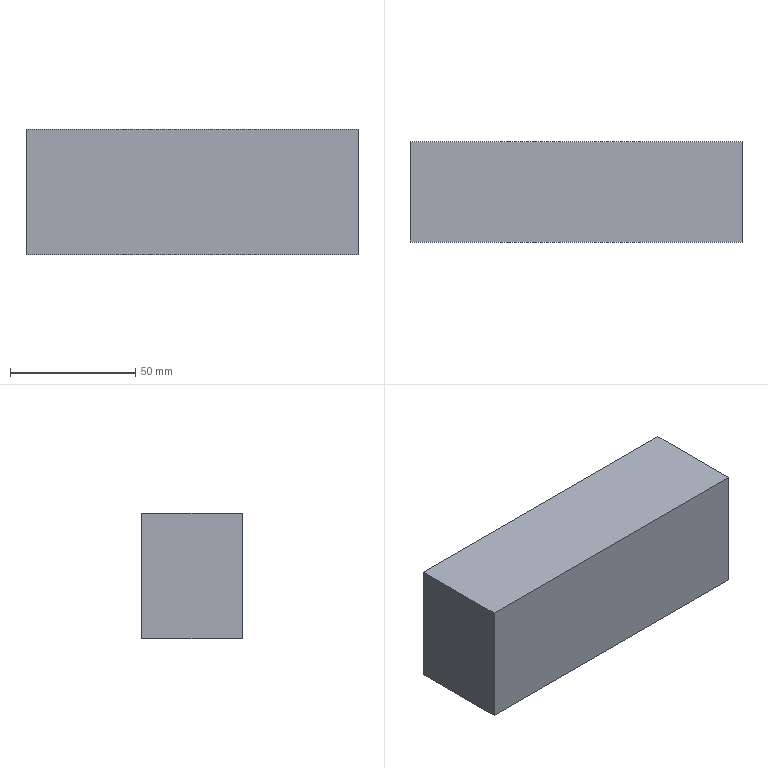Part | NX | features solid 2 | 1 solid | 6 faces | box 132.5 x 40 x 50 mm | volume 265000 mm3 | plane 4 | spline 2
STEP:
#1=CARTESIAN_POINT('',(402.5,390.,70.));
#2=VERTEX_POINT('',#1);
#3=CARTESIAN_POINT('',(270.,390.,70.));
#4=VERTEX_POINT('',#3);
#5=CARTESIAN_POINT('',(402.5,390.,70.));
#6=CARTESIAN_POINT('',(358.333,390.,70.));
#7=CARTESIAN_POINT('',(314.167,390.,70.));
#8=CARTESIAN_POINT('',(270.,390.,70.));
#9=B_SPLINE_CURVE_WITH_KNOTS('',3,(#5,#6,#7,#8),.UNSPECIFIED.,.F.,.F.,(4,4),(0.8545,0.987),.UNSPECIFIED.);
#10=EDGE_CURVE('',#2,#4,#9,.T.);
#11=ORIENTED_EDGE('',*,*,#10,.F.);
#12=CARTESIAN_POINT('',(402.5,390.,20.));
#13=VERTEX_POINT('',#12);
#14=CARTESIAN_POINT('',(402.5,390.,20.));
#15=DIRECTION('',(0.,0.,1.));
#16=VECTOR('',#15,1000.);
#17=LINE('',#14,#16);
#18=EDGE_CURVE('',#13,#2,#17,.T.);
#19=ORIENTED_EDGE('',*,*,#18,.F.);
#20=CARTESIAN_POINT('',(270.,390.,20.));
#21=VERTEX_POINT('',#20);
#22=CARTESIAN_POINT('',(402.5,390.,20.));
#23=CARTESIAN_POINT('',(358.333,390.,20.));
#24=CARTESIAN_POINT('',(314.167,390.,20.));
#25=CARTESIAN_POINT('',(270.,390.,20.));
#26=B_SPLINE_CURVE_WITH_KNOTS('',3,(#22,#23,#24,#25),.UNSPECIFIED.,.F.,.F.,(4,4),(0.8545,0.987),.UNSPECIFIED.);
#27=EDGE_CURVE('',#13,#21,#26,.T.);
#28=ORIENTED_EDGE('',*,*,#27,.T.);
#29=CARTESIAN_POINT('',(270.,390.,20.));
#30=DIRECTION('',(0.,0.,1.));
#31=VECTOR('',#30,1000.);
#32=LINE('',#29,#31);
#33=EDGE_CURVE('',#21,#4,#32,.T.);
#34=ORIENTED_EDGE('',*,*,#33,.T.);
#35=EDGE_LOOP('',(#11,#19,#28,#34));
#36=FACE_BOUND('',#35,.T.);
#37=CARTESIAN_POINT('',(442.5,390.,20.));
#38=DIRECTION('',(0.,1.,0.));
#39=DIRECTION('',(-1.,0.,0.));
#40=AXIS2_PLACEMENT_3D('',#37,#38,#39);
#41=PLANE('',#40);
#42=ADVANCED_FACE('',(#36),#41,.T.);
#43=CARTESIAN_POINT('',(270.,350.,70.));
#44=VERTEX_POINT('',#43);
#45=CARTESIAN_POINT('',(270.,490.534,70.));
#46=DIRECTION('',(0.,-1.,0.));
#47=VECTOR('',#46,1000.);
#48=LINE('',#45,#47);
#49=EDGE_CURVE('',#4,#44,#48,.T.);
#50=ORIENTED_EDGE('',*,*,#49,.F.);
#51=ORIENTED_EDGE('',*,*,#33,.F.);
#52=CARTESIAN_POINT('',(270.,350.,20.));
#53=VERTEX_POINT('',#52);
#54=CARTESIAN_POINT('',(270.,490.534,20.));
#55=DIRECTION('',(0.,-1.,0.));
#56=VECTOR('',#55,1000.);
#57=LINE('',#54,#56);
#58=EDGE_CURVE('',#21,#53,#57,.T.);
#59=ORIENTED_EDGE('',*,*,#58,.T.);
#60=CARTESIAN_POINT('',(270.,350.,20.));
#61=DIRECTION('',(0.,0.,1.));
#62=VECTOR('',#61,1000.);
#63=LINE('',#60,#62);
#64=EDGE_CURVE('',#53,#44,#63,.T.);
#65=ORIENTED_EDGE('',*,*,#64,.T.);
#66=EDGE_LOOP('',(#50,#51,#59,#65));
#67=FACE_BOUND('',#66,.T.);
#68=CARTESIAN_POINT('',(270.,490.534,20.));
#69=DIRECTION('',(-1.,0.,0.));
#70=DIRECTION('',(0.,0.,1.));
#71=AXIS2_PLACEMENT_3D('',#68,#69,#70);
#72=PLANE('',#71);
#73=ADVANCED_FACE('',(#67),#72,.T.);
#74=CARTESIAN_POINT('',(402.5,350.,70.));
#75=VERTEX_POINT('',#74);
#76=CARTESIAN_POINT('',(270.,350.,70.));
#77=CARTESIAN_POINT('',(314.167,350.,70.));
#78=CARTESIAN_POINT('',(358.333,350.,70.));
#79=CARTESIAN_POINT('',(402.5,350.,70.));
#80=B_SPLINE_CURVE_WITH_KNOTS('',3,(#76,#77,#78,#79),.UNSPECIFIED.,.F.,.F.,(4,4),(2.79,2.922),.UNSPECIFIED.);
#81=EDGE_CURVE('',#75,#44,#80,.F.);
#82=ORIENTED_EDGE('',*,*,#81,.T.);
#83=ORIENTED_EDGE('',*,*,#64,.F.);
#84=CARTESIAN_POINT('',(402.5,350.,20.));
#85=VERTEX_POINT('',#84);
#86=CARTESIAN_POINT('',(270.,350.,20.));
#87=CARTESIAN_POINT('',(314.167,350.,20.));
#88=CARTESIAN_POINT('',(358.333,350.,20.));
#89=CARTESIAN_POINT('',(402.5,350.,20.));
#90=B_SPLINE_CURVE_WITH_KNOTS('',3,(#86,#87,#88,#89),.UNSPECIFIED.,.F.,.F.,(4,4),(2.79,2.922),.UNSPECIFIED.);
#91=EDGE_CURVE('',#85,#53,#90,.F.);
#92=ORIENTED_EDGE('',*,*,#91,.F.);
#93=CARTESIAN_POINT('',(402.5,350.,20.));
#94=DIRECTION('',(0.,0.,1.));
#95=VECTOR('',#94,1000.);
#96=LINE('',#93,#95);
#97=EDGE_CURVE('',#85,#75,#96,.T.);
#98=ORIENTED_EDGE('',*,*,#97,.T.);
#99=EDGE_LOOP('',(#82,#83,#92,#98));
#100=FACE_BOUND('',#99,.T.);
#101=CARTESIAN_POINT('',(-270.,350.,20.));
#102=DIRECTION('',(0.,1.,0.));
#103=DIRECTION('',(0.,0.,1.));
#104=AXIS2_PLACEMENT_3D('',#101,#102,#103);
#105=PLANE('',#104);
#106=ADVANCED_FACE('',(#100),#105,.F.);
#107=CARTESIAN_POINT('',(402.5,350.,70.));
#108=CARTESIAN_POINT('',(402.5,363.333,70.));
#109=CARTESIAN_POINT('',(402.5,376.667,70.));
#110=CARTESIAN_POINT('',(402.5,390.,70.));
#111=B_SPLINE_CURVE_WITH_KNOTS('',3,(#107,#108,#109,#110),.UNSPECIFIED.,.F.,.F.,(4,4),(0.4214,0.4614),.UNSPECIFIED.);
#112=EDGE_CURVE('',#75,#2,#111,.T.);
#113=ORIENTED_EDGE('',*,*,#112,.F.);
#114=ORIENTED_EDGE('',*,*,#97,.F.);
#115=CARTESIAN_POINT('',(402.5,350.,20.));
#116=CARTESIAN_POINT('',(402.5,363.333,20.));
#117=CARTESIAN_POINT('',(402.5,376.667,20.));
#118=CARTESIAN_POINT('',(402.5,390.,20.));
#119=B_SPLINE_CURVE_WITH_KNOTS('',3,(#115,#116,#117,#118),.UNSPECIFIED.,.F.,.F.,(4,4),(0.4214,0.4614),.UNSPECIFIED.);
#120=EDGE_CURVE('',#85,#13,#119,.T.);
#121=ORIENTED_EDGE('',*,*,#120,.T.);
#122=ORIENTED_EDGE('',*,*,#18,.T.);
#123=EDGE_LOOP('',(#113,#114,#121,#122));
#124=FACE_BOUND('',#123,.T.);
#125=CARTESIAN_POINT('',(402.5,259.64,20.));
#126=DIRECTION('',(1.,0.,0.));
#127=DIRECTION('',(0.,0.,-1.));
#128=AXIS2_PLACEMENT_3D('',#125,#126,#127);
#129=PLANE('',#128);
#130=ADVANCED_FACE('',(#124),#129,.T.);
#131=ORIENTED_EDGE('',*,*,#27,.F.);
#132=ORIENTED_EDGE('',*,*,#120,.F.);
#133=ORIENTED_EDGE('',*,*,#91,.T.);
#134=ORIENTED_EDGE('',*,*,#58,.F.);
#135=EDGE_LOOP('',(#131,#132,#133,#134));
#136=FACE_BOUND('',#135,.T.);
#137=CARTESIAN_POINT('',(402.5,350.,20.));
#138=CARTESIAN_POINT('',(280.,350.,20.));
#139=CARTESIAN_POINT('',(270.,350.,20.));
#140=CARTESIAN_POINT('',(402.5,390.,20.));
#141=CARTESIAN_POINT('',(280.,390.,20.));
#142=CARTESIAN_POINT('',(270.,390.,20.));
#143=B_SPLINE_SURFACE_WITH_KNOTS('',1,1,((#137,#138,#139),(#140,#141,#142)),.PLANE_SURF.,.F.,.F.,.F.,(2,2),(2,1,2),(0.1041,0.2082),(-0.2188,0.,0.01786),.PIECEWISE_BEZIER_KNOTS.);
#144=ADVANCED_FACE('',(#136),#143,.F.);
#145=ORIENTED_EDGE('',*,*,#10,.T.);
#146=ORIENTED_EDGE('',*,*,#49,.T.);
#147=ORIENTED_EDGE('',*,*,#81,.F.);
#148=ORIENTED_EDGE('',*,*,#112,.T.);
#149=EDGE_LOOP('',(#145,#146,#147,#148));
#150=FACE_BOUND('',#149,.T.);
#151=CARTESIAN_POINT('',(402.5,350.,70.));
#152=CARTESIAN_POINT('',(280.,350.,70.));
#153=CARTESIAN_POINT('',(270.,350.,70.));
#154=CARTESIAN_POINT('',(402.5,390.,70.));
#155=CARTESIAN_POINT('',(280.,390.,70.));
#156=CARTESIAN_POINT('',(270.,390.,70.));
#157=B_SPLINE_SURFACE_WITH_KNOTS('',1,1,((#151,#152,#153),(#154,#155,#156)),.PLANE_SURF.,.F.,.F.,.F.,(2,2),(2,1,2),(0.1041,0.2082),(-0.2188,0.,0.01786),.PIECEWISE_BEZIER_KNOTS.);
#158=ADVANCED_FACE('',(#150),#157,.T.);
#159=CLOSED_SHELL('',(#42,#73,#106,#130,#144,#158));
#160=MANIFOLD_SOLID_BREP('',#159);
#161=(LENGTH_UNIT()NAMED_UNIT(*)SI_UNIT(.MILLI.,.METRE.));
#162=UNCERTAINTY_MEASURE_WITH_UNIT(LENGTH_MEASURE(0.0508),#161,'','');
#163=(NAMED_UNIT(*)PLANE_ANGLE_UNIT()SI_UNIT($,.RADIAN.));
#164=(NAMED_UNIT(*)SI_UNIT($,.STERADIAN.)SOLID_ANGLE_UNIT());
#165=(GEOMETRIC_REPRESENTATION_CONTEXT(3)GLOBAL_UNCERTAINTY_ASSIGNED_CONTEXT((#162))GLOBAL_UNIT_ASSIGNED_CONTEXT((#161,#163,#164))REPRESENTATION_CONTEXT('',''));
#166=ADVANCED_BREP_SHAPE_REPRESENTATION('',(#160),#165);